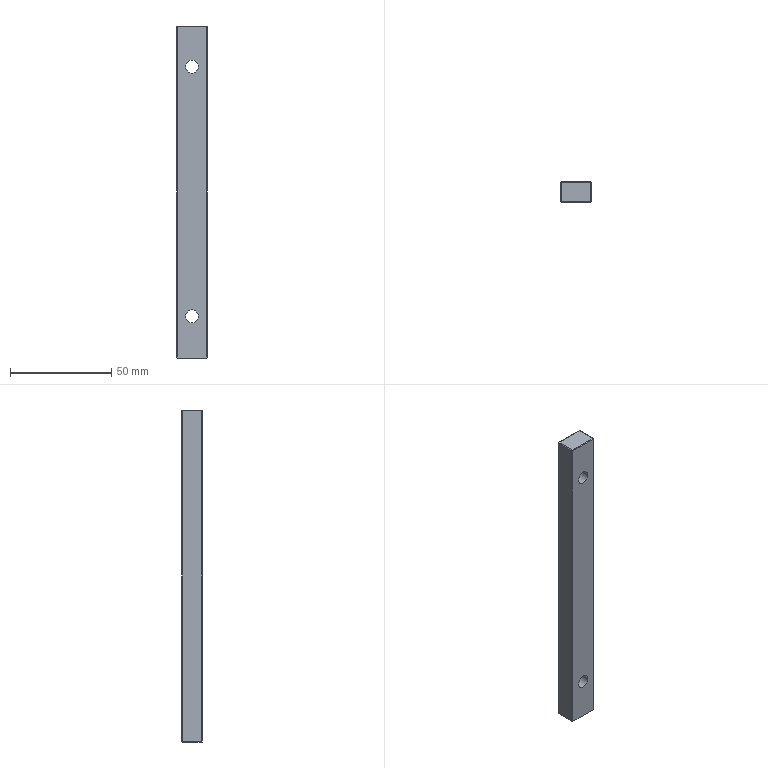Part | NX | 1 solid | 25 faces | box 15 x 10 x 164 mm | volume 23902 mm3 | plane 17 | cylinder 4 | cone 4 | commonest cylinder face diameters 6.5 x4
STEP:
#1=CARTESIAN_POINT('',(0.000000309,-112.2,61.7));
#2=VERTEX_POINT('',#1);
#3=CARTESIAN_POINT('',(0.000000309,-102.8,61.7));
#4=VERTEX_POINT('',#3);
#5=CARTESIAN_POINT('',(0.000000309,-107.5,61.7));
#6=DIRECTION('',(0.,1.,0.));
#7=VECTOR('',#6,1000.);
#8=LINE('',#5,#7);
#9=EDGE_CURVE('',#2,#4,#8,.T.);
#10=ORIENTED_EDGE('',*,*,#9,.F.);
#11=CARTESIAN_POINT('',(0.000000309,-112.2,-101.7));
#12=VERTEX_POINT('',#11);
#13=CARTESIAN_POINT('',(0.000000309,-112.2,-20.));
#14=DIRECTION('',(0.,0.,-1.));
#15=VECTOR('',#14,1000.);
#16=LINE('',#13,#15);
#17=EDGE_CURVE('',#2,#12,#16,.T.);
#18=ORIENTED_EDGE('',*,*,#17,.T.);
#19=CARTESIAN_POINT('',(0.000000309,-102.8,-101.7));
#20=VERTEX_POINT('',#19);
#21=CARTESIAN_POINT('',(0.000000309,-107.5,-101.7));
#22=DIRECTION('',(0.,-1.,0.));
#23=VECTOR('',#22,1000.);
#24=LINE('',#21,#23);
#25=EDGE_CURVE('',#20,#12,#24,.T.);
#26=ORIENTED_EDGE('',*,*,#25,.F.);
#27=CARTESIAN_POINT('',(0.000000309,-102.8,-20.));
#28=DIRECTION('',(0.,0.,1.));
#29=VECTOR('',#28,1000.);
#30=LINE('',#27,#29);
#31=EDGE_CURVE('',#20,#4,#30,.T.);
#32=ORIENTED_EDGE('',*,*,#31,.T.);
#33=EDGE_LOOP('',(#10,#18,#26,#32));
#34=FACE_BOUND('',#33,.T.);
#35=CARTESIAN_POINT('',(0.000000309,-100.5,62.));
#36=DIRECTION('',(1.,0.,0.));
#37=DIRECTION('',(0.,1.,0.));
#38=AXIS2_PLACEMENT_3D('',#35,#36,#37);
#39=PLANE('',#38);
#40=ADVANCED_FACE('',(#34),#39,.T.);
#41=CARTESIAN_POINT('',(-14.7,-102.8,62.));
#42=VERTEX_POINT('',#41);
#43=CARTESIAN_POINT('',(-14.7,-112.2,62.));
#44=VERTEX_POINT('',#43);
#45=CARTESIAN_POINT('',(-14.7,-107.5,62.));
#46=DIRECTION('',(0.,-1.,0.));
#47=VECTOR('',#46,1000.);
#48=LINE('',#45,#47);
#49=EDGE_CURVE('',#42,#44,#48,.T.);
#50=ORIENTED_EDGE('',*,*,#49,.T.);
#51=CARTESIAN_POINT('',(-0.3,-112.2,62.));
#52=VERTEX_POINT('',#51);
#53=CARTESIAN_POINT('',(-7.5,-112.2,62.));
#54=DIRECTION('',(-1.,0.,0.));
#55=VECTOR('',#54,1000.);
#56=LINE('',#53,#55);
#57=EDGE_CURVE('',#52,#44,#56,.T.);
#58=ORIENTED_EDGE('',*,*,#57,.F.);
#59=CARTESIAN_POINT('',(-0.3,-102.8,62.));
#60=VERTEX_POINT('',#59);
#61=CARTESIAN_POINT('',(-0.3,-107.5,62.));
#62=DIRECTION('',(0.,1.,0.));
#63=VECTOR('',#62,1000.);
#64=LINE('',#61,#63);
#65=EDGE_CURVE('',#52,#60,#64,.T.);
#66=ORIENTED_EDGE('',*,*,#65,.T.);
#67=CARTESIAN_POINT('',(-7.5,-102.8,62.));
#68=DIRECTION('',(-1.,0.,0.));
#69=VECTOR('',#68,1000.);
#70=LINE('',#67,#69);
#71=EDGE_CURVE('',#60,#42,#70,.T.);
#72=ORIENTED_EDGE('',*,*,#71,.T.);
#73=EDGE_LOOP('',(#50,#58,#66,#72));
#74=FACE_BOUND('',#73,.T.);
#75=CARTESIAN_POINT('',(-15.,-100.5,62.));
#76=DIRECTION('',(0.,0.,1.));
#77=DIRECTION('',(0.,-1.,0.));
#78=AXIS2_PLACEMENT_3D('',#75,#76,#77);
#79=PLANE('',#78);
#80=ADVANCED_FACE('',(#74),#79,.T.);
#81=CARTESIAN_POINT('',(-15.,-102.8,-101.7));
#82=VERTEX_POINT('',#81);
#83=CARTESIAN_POINT('',(-15.,-112.2,-101.7));
#84=VERTEX_POINT('',#83);
#85=CARTESIAN_POINT('',(-15.,-107.5,-101.7));
#86=DIRECTION('',(0.,-1.,0.));
#87=VECTOR('',#86,1000.);
#88=LINE('',#85,#87);
#89=EDGE_CURVE('',#82,#84,#88,.T.);
#90=ORIENTED_EDGE('',*,*,#89,.T.);
#91=CARTESIAN_POINT('',(-15.,-112.2,61.7));
#92=VERTEX_POINT('',#91);
#93=CARTESIAN_POINT('',(-15.,-112.2,-20.));
#94=DIRECTION('',(0.,0.,-1.));
#95=VECTOR('',#94,1000.);
#96=LINE('',#93,#95);
#97=EDGE_CURVE('',#92,#84,#96,.T.);
#98=ORIENTED_EDGE('',*,*,#97,.F.);
#99=CARTESIAN_POINT('',(-15.,-102.8,61.7));
#100=VERTEX_POINT('',#99);
#101=CARTESIAN_POINT('',(-15.,-107.5,61.7));
#102=DIRECTION('',(0.,-1.,0.));
#103=VECTOR('',#102,1000.);
#104=LINE('',#101,#103);
#105=EDGE_CURVE('',#100,#92,#104,.T.);
#106=ORIENTED_EDGE('',*,*,#105,.F.);
#107=CARTESIAN_POINT('',(-15.,-102.8,-20.));
#108=DIRECTION('',(0.,0.,-1.));
#109=VECTOR('',#108,1000.);
#110=LINE('',#107,#109);
#111=EDGE_CURVE('',#100,#82,#110,.T.);
#112=ORIENTED_EDGE('',*,*,#111,.T.);
#113=EDGE_LOOP('',(#90,#98,#106,#112));
#114=FACE_BOUND('',#113,.T.);
#115=CARTESIAN_POINT('',(-15.,-100.5,-102.));
#116=DIRECTION('',(-1.,0.,0.));
#117=DIRECTION('',(0.,0.,1.));
#118=AXIS2_PLACEMENT_3D('',#115,#116,#117);
#119=PLANE('',#118);
#120=ADVANCED_FACE('',(#114),#119,.T.);
#121=CARTESIAN_POINT('',(-14.7,-102.8,-102.));
#122=VERTEX_POINT('',#121);
#123=CARTESIAN_POINT('',(-0.3,-102.8,-102.));
#124=VERTEX_POINT('',#123);
#125=CARTESIAN_POINT('',(-7.5,-102.8,-102.));
#126=DIRECTION('',(1.,0.,0.));
#127=VECTOR('',#126,1000.);
#128=LINE('',#125,#127);
#129=EDGE_CURVE('',#122,#124,#128,.T.);
#130=ORIENTED_EDGE('',*,*,#129,.T.);
#131=CARTESIAN_POINT('',(-0.3,-112.5,-102.));
#132=VERTEX_POINT('',#131);
#133=CARTESIAN_POINT('',(-0.3,-107.5,-102.));
#134=DIRECTION('',(0.,-1.,0.));
#135=VECTOR('',#134,1000.);
#136=LINE('',#133,#135);
#137=EDGE_CURVE('',#124,#132,#136,.T.);
#138=ORIENTED_EDGE('',*,*,#137,.T.);
#139=CARTESIAN_POINT('',(-14.7,-112.5,-102.));
#140=VERTEX_POINT('',#139);
#141=CARTESIAN_POINT('',(-105.,-112.5,-102.));
#142=DIRECTION('',(1.,0.,0.));
#143=VECTOR('',#142,1000.);
#144=LINE('',#141,#143);
#145=EDGE_CURVE('',#140,#132,#144,.T.);
#146=ORIENTED_EDGE('',*,*,#145,.F.);
#147=CARTESIAN_POINT('',(-14.7,-107.5,-102.));
#148=DIRECTION('',(0.,-1.,0.));
#149=VECTOR('',#148,1000.);
#150=LINE('',#147,#149);
#151=EDGE_CURVE('',#122,#140,#150,.T.);
#152=ORIENTED_EDGE('',*,*,#151,.F.);
#153=EDGE_LOOP('',(#130,#138,#146,#152));
#154=FACE_BOUND('',#153,.T.);
#155=CARTESIAN_POINT('',(-4.,-100.5,-102.));
#156=DIRECTION('',(0.,0.,-1.));
#157=DIRECTION('',(-1.,0.,0.));
#158=AXIS2_PLACEMENT_3D('',#155,#156,#157);
#159=PLANE('',#158);
#160=ADVANCED_FACE('',(#154),#159,.T.);
#161=CARTESIAN_POINT('',(-4.25,-102.7,-81.438));
#162=VERTEX_POINT('',#161);
#163=CARTESIAN_POINT('',(-10.75,-102.7,-81.438));
#164=VERTEX_POINT('',#163);
#165=CARTESIAN_POINT('',(-7.5,-102.7,-81.438));
#166=DIRECTION('',(0.,1.,0.));
#167=DIRECTION('',(-1.,0.,0.));
#168=AXIS2_PLACEMENT_3D('',#165,#166,#167);
#169=CIRCLE('',#168,3.25);
#170=EDGE_CURVE('',#162,#164,#169,.T.);
#171=ORIENTED_EDGE('',*,*,#170,.T.);
#172=CARTESIAN_POINT('',(-10.75,-112.5,-81.438));
#173=VERTEX_POINT('',#172);
#174=CARTESIAN_POINT('',(-10.75,-102.5,-81.438));
#175=DIRECTION('',(0.,1.,0.));
#176=VECTOR('',#175,1000.);
#177=LINE('',#174,#176);
#178=EDGE_CURVE('',#164,#173,#177,.F.);
#179=ORIENTED_EDGE('',*,*,#178,.T.);
#180=CARTESIAN_POINT('',(-4.25,-112.5,-81.438));
#181=VERTEX_POINT('',#180);
#182=CARTESIAN_POINT('',(-7.5,-112.5,-81.438));
#183=DIRECTION('',(0.,1.,0.));
#184=DIRECTION('',(-1.,0.,0.));
#185=AXIS2_PLACEMENT_3D('',#182,#183,#184);
#186=CIRCLE('',#185,3.25);
#187=EDGE_CURVE('',#181,#173,#186,.T.);
#188=ORIENTED_EDGE('',*,*,#187,.F.);
#189=CARTESIAN_POINT('',(-4.25,-102.5,-81.438));
#190=DIRECTION('',(0.,1.,0.));
#191=VECTOR('',#190,1000.);
#192=LINE('',#189,#191);
#193=EDGE_CURVE('',#162,#181,#192,.F.);
#194=ORIENTED_EDGE('',*,*,#193,.F.);
#195=EDGE_LOOP('',(#171,#179,#188,#194));
#196=FACE_BOUND('',#195,.T.);
#197=CARTESIAN_POINT('',(-7.5,-102.5,-81.438));
#198=DIRECTION('',(0.,1.,0.));
#199=DIRECTION('',(-1.,0.,0.));
#200=AXIS2_PLACEMENT_3D('',#197,#198,#199);
#201=CYLINDRICAL_SURFACE('',#200,3.25);
#202=ADVANCED_FACE('',(#196),#201,.F.);
#203=ORIENTED_EDGE('',*,*,#170,.F.);
#204=CARTESIAN_POINT('',(-4.05,-102.5,-81.438));
#205=VERTEX_POINT('',#204);
#206=CARTESIAN_POINT('',(-4.25,-102.7,-81.438));
#207=DIRECTION('',(0.7071,0.7071,0.));
#208=VECTOR('',#207,1000.);
#209=LINE('',#206,#208);
#210=EDGE_CURVE('',#205,#162,#209,.F.);
#211=ORIENTED_EDGE('',*,*,#210,.F.);
#212=CARTESIAN_POINT('',(-10.95,-102.5,-81.438));
#213=VERTEX_POINT('',#212);
#214=CARTESIAN_POINT('',(-7.5,-102.5,-81.438));
#215=DIRECTION('',(0.,1.,0.));
#216=DIRECTION('',(-1.,0.,0.));
#217=AXIS2_PLACEMENT_3D('',#214,#215,#216);
#218=CIRCLE('',#217,3.45);
#219=EDGE_CURVE('',#205,#213,#218,.T.);
#220=ORIENTED_EDGE('',*,*,#219,.T.);
#221=CARTESIAN_POINT('',(-10.75,-102.7,-81.438));
#222=DIRECTION('',(-0.7071,0.7071,0.));
#223=VECTOR('',#222,1000.);
#224=LINE('',#221,#223);
#225=EDGE_CURVE('',#213,#164,#224,.F.);
#226=ORIENTED_EDGE('',*,*,#225,.T.);
#227=EDGE_LOOP('',(#203,#211,#220,#226));
#228=FACE_BOUND('',#227,.T.);
#229=CARTESIAN_POINT('',(-7.5,-102.7,-81.438));
#230=DIRECTION('',(0.,1.,0.));
#231=DIRECTION('',(-1.,0.,0.));
#232=AXIS2_PLACEMENT_3D('',#229,#230,#231);
#233=CONICAL_SURFACE('',#232,3.25,0.7854);
#234=ADVANCED_FACE('',(#228),#233,.F.);
#235=ORIENTED_EDGE('',*,*,#89,.F.);
#236=CARTESIAN_POINT('',(-14.85,-102.65,-101.85));
#237=VERTEX_POINT('',#236);
#238=CARTESIAN_POINT('',(-12.7,-100.5,-104.));
#239=DIRECTION('',(0.5774,0.5774,-0.5774));
#240=VECTOR('',#239,1000.);
#241=LINE('',#238,#240);
#242=EDGE_CURVE('',#82,#237,#241,.T.);
#243=ORIENTED_EDGE('',*,*,#242,.T.);
#244=CARTESIAN_POINT('',(-17.,-100.5,-99.7));
#245=DIRECTION('',(0.5774,-0.5774,-0.5774));
#246=VECTOR('',#245,1000.);
#247=LINE('',#244,#246);
#248=EDGE_CURVE('',#237,#122,#247,.T.);
#249=ORIENTED_EDGE('',*,*,#248,.T.);
#250=ORIENTED_EDGE('',*,*,#151,.T.);
#251=CARTESIAN_POINT('',(-26.7,-100.5,-90.));
#252=DIRECTION('',(-0.5774,0.5774,0.5774));
#253=VECTOR('',#252,1000.);
#254=LINE('',#251,#253);
#255=EDGE_CURVE('',#140,#84,#254,.T.);
#256=ORIENTED_EDGE('',*,*,#255,.T.);
#257=EDGE_LOOP('',(#235,#243,#249,#250,#256));
#258=FACE_BOUND('',#257,.T.);
#259=CARTESIAN_POINT('',(-14.85,-107.5,-101.85));
#260=DIRECTION('',(-0.7071,0.,-0.7071));
#261=DIRECTION('',(-0.7071,0.,0.7071));
#262=AXIS2_PLACEMENT_3D('',#259,#260,#261);
#263=PLANE('',#262);
#264=ADVANCED_FACE('',(#258),#263,.T.);
#265=ORIENTED_EDGE('',*,*,#25,.T.);
#266=CARTESIAN_POINT('',(81.95,-30.25,-19.75));
#267=DIRECTION('',(-0.5774,-0.5774,-0.5774));
#268=VECTOR('',#267,1000.);
#269=LINE('',#266,#268);
#270=EDGE_CURVE('',#12,#132,#269,.T.);
#271=ORIENTED_EDGE('',*,*,#270,.T.);
#272=ORIENTED_EDGE('',*,*,#137,.F.);
#273=CARTESIAN_POINT('',(-0.15,-102.65,-101.85));
#274=VERTEX_POINT('',#273);
#275=CARTESIAN_POINT('',(2.,-100.5,-99.7));
#276=DIRECTION('',(-0.5774,-0.5774,-0.5774));
#277=VECTOR('',#276,1000.);
#278=LINE('',#275,#277);
#279=EDGE_CURVE('',#274,#124,#278,.T.);
#280=ORIENTED_EDGE('',*,*,#279,.F.);
#281=CARTESIAN_POINT('',(81.95,-184.75,-19.75));
#282=DIRECTION('',(0.5774,-0.5774,0.5774));
#283=VECTOR('',#282,1000.);
#284=LINE('',#281,#283);
#285=EDGE_CURVE('',#274,#20,#284,.T.);
#286=ORIENTED_EDGE('',*,*,#285,.T.);
#287=EDGE_LOOP('',(#265,#271,#272,#280,#286));
#288=FACE_BOUND('',#287,.T.);
#289=CARTESIAN_POINT('',(-0.15,-107.5,-101.85));
#290=DIRECTION('',(-0.7071,0.,0.7071));
#291=DIRECTION('',(0.,1.,0.));
#292=AXIS2_PLACEMENT_3D('',#289,#290,#291);
#293=PLANE('',#292);
#294=ADVANCED_FACE('',(#288),#293,.F.);
#295=ORIENTED_EDGE('',*,*,#49,.F.);
#296=CARTESIAN_POINT('',(-14.85,-102.65,61.85));
#297=VERTEX_POINT('',#296);
#298=CARTESIAN_POINT('',(-17.,-100.5,59.7));
#299=DIRECTION('',(0.5774,-0.5774,0.5774));
#300=VECTOR('',#299,1000.);
#301=LINE('',#298,#300);
#302=EDGE_CURVE('',#297,#42,#301,.T.);
#303=ORIENTED_EDGE('',*,*,#302,.F.);
#304=CARTESIAN_POINT('',(-96.45,-184.25,-19.75));
#305=DIRECTION('',(-0.5774,-0.5774,-0.5774));
#306=VECTOR('',#305,1000.);
#307=LINE('',#304,#306);
#308=EDGE_CURVE('',#297,#100,#307,.T.);
#309=ORIENTED_EDGE('',*,*,#308,.T.);
#310=ORIENTED_EDGE('',*,*,#105,.T.);
#311=CARTESIAN_POINT('',(-14.85,-112.35,61.85));
#312=VERTEX_POINT('',#311);
#313=CARTESIAN_POINT('',(-96.45,-30.75,-19.75));
#314=DIRECTION('',(-0.5774,0.5774,-0.5774));
#315=VECTOR('',#314,1000.);
#316=LINE('',#313,#315);
#317=EDGE_CURVE('',#312,#92,#316,.T.);
#318=ORIENTED_EDGE('',*,*,#317,.F.);
#319=CARTESIAN_POINT('',(-3.,-100.5,73.7));
#320=DIRECTION('',(0.5774,0.5774,0.5774));
#321=VECTOR('',#320,1000.);
#322=LINE('',#319,#321);
#323=EDGE_CURVE('',#312,#44,#322,.T.);
#324=ORIENTED_EDGE('',*,*,#323,.T.);
#325=EDGE_LOOP('',(#295,#303,#309,#310,#318,#324));
#326=FACE_BOUND('',#325,.T.);
#327=CARTESIAN_POINT('',(-14.85,-107.5,61.85));
#328=DIRECTION('',(-0.7071,0.,0.7071));
#329=DIRECTION('',(0.,1.,0.));
#330=AXIS2_PLACEMENT_3D('',#327,#328,#329);
#331=PLANE('',#330);
#332=ADVANCED_FACE('',(#326),#331,.T.);
#333=ORIENTED_EDGE('',*,*,#9,.T.);
#334=CARTESIAN_POINT('',(-0.15,-102.65,61.85));
#335=VERTEX_POINT('',#334);
#336=CARTESIAN_POINT('',(-2.3,-100.5,64.));
#337=DIRECTION('',(0.5774,-0.5774,-0.5774));
#338=VECTOR('',#337,1000.);
#339=LINE('',#336,#338);
#340=EDGE_CURVE('',#335,#4,#339,.T.);
#341=ORIENTED_EDGE('',*,*,#340,.F.);
#342=CARTESIAN_POINT('',(2.,-100.5,59.7));
#343=DIRECTION('',(0.5774,0.5774,-0.5774));
#344=VECTOR('',#343,1000.);
#345=LINE('',#342,#344);
#346=EDGE_CURVE('',#60,#335,#345,.T.);
#347=ORIENTED_EDGE('',*,*,#346,.F.);
#348=ORIENTED_EDGE('',*,*,#65,.F.);
#349=CARTESIAN_POINT('',(-0.15,-112.35,61.85));
#350=VERTEX_POINT('',#349);
#351=CARTESIAN_POINT('',(-12.,-100.5,73.7));
#352=DIRECTION('',(-0.5774,0.5774,0.5774));
#353=VECTOR('',#352,1000.);
#354=LINE('',#351,#353);
#355=EDGE_CURVE('',#350,#52,#354,.T.);
#356=ORIENTED_EDGE('',*,*,#355,.F.);
#357=CARTESIAN_POINT('',(11.7,-100.5,50.));
#358=DIRECTION('',(-0.5774,-0.5774,0.5774));
#359=VECTOR('',#358,1000.);
#360=LINE('',#357,#359);
#361=EDGE_CURVE('',#2,#350,#360,.T.);
#362=ORIENTED_EDGE('',*,*,#361,.F.);
#363=EDGE_LOOP('',(#333,#341,#347,#348,#356,#362));
#364=FACE_BOUND('',#363,.T.);
#365=CARTESIAN_POINT('',(-0.15,-107.5,61.85));
#366=DIRECTION('',(-0.7071,0.,-0.7071));
#367=DIRECTION('',(-0.7071,0.,0.7071));
#368=AXIS2_PLACEMENT_3D('',#365,#366,#367);
#369=PLANE('',#368);
#370=ADVANCED_FACE('',(#364),#369,.F.);
#371=ORIENTED_EDGE('',*,*,#178,.F.);
#372=CARTESIAN_POINT('',(-7.5,-102.7,-81.438));
#373=DIRECTION('',(0.,1.,0.));
#374=DIRECTION('',(-1.,0.,0.));
#375=AXIS2_PLACEMENT_3D('',#372,#373,#374);
#376=CIRCLE('',#375,3.25);
#377=EDGE_CURVE('',#164,#162,#376,.T.);
#378=ORIENTED_EDGE('',*,*,#377,.T.);
#379=ORIENTED_EDGE('',*,*,#193,.T.);
#380=CARTESIAN_POINT('',(-7.5,-112.5,-81.438));
#381=DIRECTION('',(0.,1.,0.));
#382=DIRECTION('',(-1.,0.,0.));
#383=AXIS2_PLACEMENT_3D('',#380,#381,#382);
#384=CIRCLE('',#383,3.25);
#385=EDGE_CURVE('',#173,#181,#384,.T.);
#386=ORIENTED_EDGE('',*,*,#385,.F.);
#387=EDGE_LOOP('',(#371,#378,#379,#386));
#388=FACE_BOUND('',#387,.T.);
#389=CARTESIAN_POINT('',(-7.5,-102.5,-81.438));
#390=DIRECTION('',(0.,1.,0.));
#391=DIRECTION('',(-1.,0.,0.));
#392=AXIS2_PLACEMENT_3D('',#389,#390,#391);
#393=CYLINDRICAL_SURFACE('',#392,3.25);
#394=ADVANCED_FACE('',(#388),#393,.F.);
#395=ORIENTED_EDGE('',*,*,#225,.F.);
#396=CARTESIAN_POINT('',(-7.5,-102.5,-81.438));
#397=DIRECTION('',(0.,1.,0.));
#398=DIRECTION('',(-1.,0.,0.));
#399=AXIS2_PLACEMENT_3D('',#396,#397,#398);
#400=CIRCLE('',#399,3.45);
#401=EDGE_CURVE('',#213,#205,#400,.T.);
#402=ORIENTED_EDGE('',*,*,#401,.T.);
#403=ORIENTED_EDGE('',*,*,#210,.T.);
#404=ORIENTED_EDGE('',*,*,#377,.F.);
#405=EDGE_LOOP('',(#395,#402,#403,#404));
#406=FACE_BOUND('',#405,.T.);
#407=CARTESIAN_POINT('',(-7.5,-102.7,-81.438));
#408=DIRECTION('',(0.,1.,0.));
#409=DIRECTION('',(-1.,0.,0.));
#410=AXIS2_PLACEMENT_3D('',#407,#408,#409);
#411=CONICAL_SURFACE('',#410,3.25,0.7854);
#412=ADVANCED_FACE('',(#406),#411,.F.);
#413=CARTESIAN_POINT('',(-0.3,-112.5,61.7));
#414=VERTEX_POINT('',#413);
#415=CARTESIAN_POINT('',(-14.7,-112.5,61.7));
#416=VERTEX_POINT('',#415);
#417=CARTESIAN_POINT('',(-7.5,-112.5,61.7));
#418=DIRECTION('',(-1.,0.,0.));
#419=VECTOR('',#418,1000.);
#420=LINE('',#417,#419);
#421=EDGE_CURVE('',#414,#416,#420,.T.);
#422=ORIENTED_EDGE('',*,*,#421,.T.);
#423=CARTESIAN_POINT('',(-14.7,-112.5,-20.));
#424=DIRECTION('',(0.,0.,-1.));
#425=VECTOR('',#424,1000.);
#426=LINE('',#423,#425);
#427=EDGE_CURVE('',#416,#140,#426,.T.);
#428=ORIENTED_EDGE('',*,*,#427,.T.);
#429=ORIENTED_EDGE('',*,*,#145,.T.);
#430=CARTESIAN_POINT('',(-0.3,-112.5,-20.));
#431=DIRECTION('',(0.,0.,-1.));
#432=VECTOR('',#431,1000.);
#433=LINE('',#430,#432);
#434=EDGE_CURVE('',#414,#132,#433,.T.);
#435=ORIENTED_EDGE('',*,*,#434,.F.);
#436=EDGE_LOOP('',(#422,#428,#429,#435));
#437=FACE_BOUND('',#436,.T.);
#438=ORIENTED_EDGE('',*,*,#187,.T.);
#439=ORIENTED_EDGE('',*,*,#385,.T.);
#440=EDGE_LOOP('',(#438,#439));
#441=FACE_BOUND('',#440,.T.);
#442=CARTESIAN_POINT('',(-4.25,-112.5,41.937));
#443=VERTEX_POINT('',#442);
#444=CARTESIAN_POINT('',(-10.75,-112.5,41.937));
#445=VERTEX_POINT('',#444);
#446=CARTESIAN_POINT('',(-7.5,-112.5,41.937));
#447=DIRECTION('',(0.,1.,0.));
#448=DIRECTION('',(-1.,0.,0.));
#449=AXIS2_PLACEMENT_3D('',#446,#447,#448);
#450=CIRCLE('',#449,3.25);
#451=EDGE_CURVE('',#443,#445,#450,.T.);
#452=ORIENTED_EDGE('',*,*,#451,.T.);
#453=CARTESIAN_POINT('',(-7.5,-112.5,41.937));
#454=DIRECTION('',(0.,1.,0.));
#455=DIRECTION('',(-1.,0.,0.));
#456=AXIS2_PLACEMENT_3D('',#453,#454,#455);
#457=CIRCLE('',#456,3.25);
#458=EDGE_CURVE('',#445,#443,#457,.T.);
#459=ORIENTED_EDGE('',*,*,#458,.T.);
#460=EDGE_LOOP('',(#452,#459));
#461=FACE_BOUND('',#460,.T.);
#462=CARTESIAN_POINT('',(-105.,-112.5,-19.75));
#463=DIRECTION('',(0.,1.,0.));
#464=DIRECTION('',(0.,0.,-1.));
#465=AXIS2_PLACEMENT_3D('',#462,#463,#464);
#466=PLANE('',#465);
#467=ADVANCED_FACE('',(#437,#441,#461),#466,.F.);
#468=CARTESIAN_POINT('',(-4.25,-102.7,41.937));
#469=VERTEX_POINT('',#468);
#470=CARTESIAN_POINT('',(-10.75,-102.7,41.937));
#471=VERTEX_POINT('',#470);
#472=CARTESIAN_POINT('',(-7.5,-102.7,41.937));
#473=DIRECTION('',(0.,1.,0.));
#474=DIRECTION('',(-1.,0.,0.));
#475=AXIS2_PLACEMENT_3D('',#472,#473,#474);
#476=CIRCLE('',#475,3.25);
#477=EDGE_CURVE('',#469,#471,#476,.T.);
#478=ORIENTED_EDGE('',*,*,#477,.T.);
#479=CARTESIAN_POINT('',(-10.75,-102.5,41.937));
#480=DIRECTION('',(0.,1.,0.));
#481=VECTOR('',#480,1000.);
#482=LINE('',#479,#481);
#483=EDGE_CURVE('',#471,#445,#482,.F.);
#484=ORIENTED_EDGE('',*,*,#483,.T.);
#485=ORIENTED_EDGE('',*,*,#451,.F.);
#486=CARTESIAN_POINT('',(-4.25,-102.5,41.937));
#487=DIRECTION('',(0.,1.,0.));
#488=VECTOR('',#487,1000.);
#489=LINE('',#486,#488);
#490=EDGE_CURVE('',#469,#443,#489,.F.);
#491=ORIENTED_EDGE('',*,*,#490,.F.);
#492=EDGE_LOOP('',(#478,#484,#485,#491));
#493=FACE_BOUND('',#492,.T.);
#494=CARTESIAN_POINT('',(-7.5,-102.5,41.937));
#495=DIRECTION('',(0.,1.,0.));
#496=DIRECTION('',(-1.,0.,0.));
#497=AXIS2_PLACEMENT_3D('',#494,#495,#496);
#498=CYLINDRICAL_SURFACE('',#497,3.25);
#499=ADVANCED_FACE('',(#493),#498,.F.);
#500=ORIENTED_EDGE('',*,*,#477,.F.);
#501=CARTESIAN_POINT('',(-4.05,-102.5,41.937));
#502=VERTEX_POINT('',#501);
#503=CARTESIAN_POINT('',(-4.25,-102.7,41.937));
#504=DIRECTION('',(0.7071,0.7071,0.));
#505=VECTOR('',#504,1000.);
#506=LINE('',#503,#505);
#507=EDGE_CURVE('',#502,#469,#506,.F.);
#508=ORIENTED_EDGE('',*,*,#507,.F.);
#509=CARTESIAN_POINT('',(-10.95,-102.5,41.937));
#510=VERTEX_POINT('',#509);
#511=CARTESIAN_POINT('',(-7.5,-102.5,41.937));
#512=DIRECTION('',(0.,1.,0.));
#513=DIRECTION('',(-1.,0.,0.));
#514=AXIS2_PLACEMENT_3D('',#511,#512,#513);
#515=CIRCLE('',#514,3.45);
#516=EDGE_CURVE('',#502,#510,#515,.T.);
#517=ORIENTED_EDGE('',*,*,#516,.T.);
#518=CARTESIAN_POINT('',(-10.75,-102.7,41.937));
#519=DIRECTION('',(-0.7071,0.7071,0.));
#520=VECTOR('',#519,1000.);
#521=LINE('',#518,#520);
#522=EDGE_CURVE('',#510,#471,#521,.F.);
#523=ORIENTED_EDGE('',*,*,#522,.T.);
#524=EDGE_LOOP('',(#500,#508,#517,#523));
#525=FACE_BOUND('',#524,.T.);
#526=CARTESIAN_POINT('',(-7.5,-102.7,41.937));
#527=DIRECTION('',(0.,1.,0.));
#528=DIRECTION('',(-1.,0.,0.));
#529=AXIS2_PLACEMENT_3D('',#526,#527,#528);
#530=CONICAL_SURFACE('',#529,3.25,0.7854);
#531=ADVANCED_FACE('',(#525),#530,.F.);
#532=ORIENTED_EDGE('',*,*,#427,.F.);
#533=CARTESIAN_POINT('',(-26.7,-100.5,73.7));
#534=DIRECTION('',(-0.5774,0.5774,0.5774));
#535=VECTOR('',#534,1000.);
#536=LINE('',#533,#535);
#537=EDGE_CURVE('',#416,#312,#536,.T.);
#538=ORIENTED_EDGE('',*,*,#537,.T.);
#539=ORIENTED_EDGE('',*,*,#317,.T.);
#540=ORIENTED_EDGE('',*,*,#97,.T.);
#541=ORIENTED_EDGE('',*,*,#255,.F.);
#542=EDGE_LOOP('',(#532,#538,#539,#540,#541));
#543=FACE_BOUND('',#542,.T.);
#544=CARTESIAN_POINT('',(-14.85,-112.35,-20.));
#545=DIRECTION('',(-0.7071,-0.7071,0.));
#546=DIRECTION('',(-0.7071,0.7071,0.));
#547=AXIS2_PLACEMENT_3D('',#544,#545,#546);
#548=PLANE('',#547);
#549=ADVANCED_FACE('',(#543),#548,.T.);
#550=ORIENTED_EDGE('',*,*,#434,.T.);
#551=ORIENTED_EDGE('',*,*,#270,.F.);
#552=ORIENTED_EDGE('',*,*,#17,.F.);
#553=ORIENTED_EDGE('',*,*,#361,.T.);
#554=CARTESIAN_POINT('',(11.7,-100.5,73.7));
#555=DIRECTION('',(0.5774,0.5774,0.5774));
#556=VECTOR('',#555,1000.);
#557=LINE('',#554,#556);
#558=EDGE_CURVE('',#414,#350,#557,.T.);
#559=ORIENTED_EDGE('',*,*,#558,.F.);
#560=EDGE_LOOP('',(#550,#551,#552,#553,#559));
#561=FACE_BOUND('',#560,.T.);
#562=CARTESIAN_POINT('',(-0.15,-112.35,-20.));
#563=DIRECTION('',(-0.7071,0.7071,0.));
#564=DIRECTION('',(0.,0.,1.));
#565=AXIS2_PLACEMENT_3D('',#562,#563,#564);
#566=PLANE('',#565);
#567=ADVANCED_FACE('',(#561),#566,.F.);
#568=ORIENTED_EDGE('',*,*,#421,.F.);
#569=ORIENTED_EDGE('',*,*,#558,.T.);
#570=ORIENTED_EDGE('',*,*,#355,.T.);
#571=ORIENTED_EDGE('',*,*,#57,.T.);
#572=ORIENTED_EDGE('',*,*,#323,.F.);
#573=ORIENTED_EDGE('',*,*,#537,.F.);
#574=EDGE_LOOP('',(#568,#569,#570,#571,#572,#573));
#575=FACE_BOUND('',#574,.T.);
#576=CARTESIAN_POINT('',(-7.5,-112.35,61.85));
#577=DIRECTION('',(0.,-0.7071,0.7071));
#578=DIRECTION('',(-1.,0.,0.));
#579=AXIS2_PLACEMENT_3D('',#576,#577,#578);
#580=PLANE('',#579);
#581=ADVANCED_FACE('',(#575),#580,.T.);
#582=ORIENTED_EDGE('',*,*,#483,.F.);
#583=CARTESIAN_POINT('',(-7.5,-102.7,41.937));
#584=DIRECTION('',(0.,1.,0.));
#585=DIRECTION('',(-1.,0.,0.));
#586=AXIS2_PLACEMENT_3D('',#583,#584,#585);
#587=CIRCLE('',#586,3.25);
#588=EDGE_CURVE('',#471,#469,#587,.T.);
#589=ORIENTED_EDGE('',*,*,#588,.T.);
#590=ORIENTED_EDGE('',*,*,#490,.T.);
#591=ORIENTED_EDGE('',*,*,#458,.F.);
#592=EDGE_LOOP('',(#582,#589,#590,#591));
#593=FACE_BOUND('',#592,.T.);
#594=CARTESIAN_POINT('',(-7.5,-102.5,41.937));
#595=DIRECTION('',(0.,1.,0.));
#596=DIRECTION('',(-1.,0.,0.));
#597=AXIS2_PLACEMENT_3D('',#594,#595,#596);
#598=CYLINDRICAL_SURFACE('',#597,3.25);
#599=ADVANCED_FACE('',(#593),#598,.F.);
#600=ORIENTED_EDGE('',*,*,#522,.F.);
#601=CARTESIAN_POINT('',(-7.5,-102.5,41.937));
#602=DIRECTION('',(0.,1.,0.));
#603=DIRECTION('',(-1.,0.,0.));
#604=AXIS2_PLACEMENT_3D('',#601,#602,#603);
#605=CIRCLE('',#604,3.45);
#606=EDGE_CURVE('',#510,#502,#605,.T.);
#607=ORIENTED_EDGE('',*,*,#606,.T.);
#608=ORIENTED_EDGE('',*,*,#507,.T.);
#609=ORIENTED_EDGE('',*,*,#588,.F.);
#610=EDGE_LOOP('',(#600,#607,#608,#609));
#611=FACE_BOUND('',#610,.T.);
#612=CARTESIAN_POINT('',(-7.5,-102.7,41.937));
#613=DIRECTION('',(0.,1.,0.));
#614=DIRECTION('',(-1.,0.,0.));
#615=AXIS2_PLACEMENT_3D('',#612,#613,#614);
#616=CONICAL_SURFACE('',#615,3.25,0.7854);
#617=ADVANCED_FACE('',(#611),#616,.F.);
#618=CARTESIAN_POINT('',(-0.3,-102.5,61.7));
#619=VERTEX_POINT('',#618);
#620=CARTESIAN_POINT('',(-14.7,-102.5,61.7));
#621=VERTEX_POINT('',#620);
#622=CARTESIAN_POINT('',(-7.5,-102.5,61.7));
#623=DIRECTION('',(-1.,0.,0.));
#624=VECTOR('',#623,1000.);
#625=LINE('',#622,#624);
#626=EDGE_CURVE('',#619,#621,#625,.T.);
#627=ORIENTED_EDGE('',*,*,#626,.F.);
#628=CARTESIAN_POINT('',(-0.3,-102.5,-101.7));
#629=VERTEX_POINT('',#628);
#630=CARTESIAN_POINT('',(-0.3,-102.5,-20.));
#631=DIRECTION('',(0.,0.,1.));
#632=VECTOR('',#631,1000.);
#633=LINE('',#630,#632);
#634=EDGE_CURVE('',#629,#619,#633,.T.);
#635=ORIENTED_EDGE('',*,*,#634,.F.);
#636=CARTESIAN_POINT('',(-14.7,-102.5,-101.7));
#637=VERTEX_POINT('',#636);
#638=CARTESIAN_POINT('',(-7.5,-102.5,-101.7));
#639=DIRECTION('',(1.,0.,0.));
#640=VECTOR('',#639,1000.);
#641=LINE('',#638,#640);
#642=EDGE_CURVE('',#637,#629,#641,.T.);
#643=ORIENTED_EDGE('',*,*,#642,.F.);
#644=CARTESIAN_POINT('',(-14.7,-102.5,-20.));
#645=DIRECTION('',(0.,0.,-1.));
#646=VECTOR('',#645,1000.);
#647=LINE('',#644,#646);
#648=EDGE_CURVE('',#621,#637,#647,.T.);
#649=ORIENTED_EDGE('',*,*,#648,.F.);
#650=EDGE_LOOP('',(#627,#635,#643,#649));
#651=FACE_BOUND('',#650,.T.);
#652=ORIENTED_EDGE('',*,*,#516,.F.);
#653=ORIENTED_EDGE('',*,*,#606,.F.);
#654=EDGE_LOOP('',(#652,#653));
#655=FACE_BOUND('',#654,.T.);
#656=ORIENTED_EDGE('',*,*,#219,.F.);
#657=ORIENTED_EDGE('',*,*,#401,.F.);
#658=EDGE_LOOP('',(#656,#657));
#659=FACE_BOUND('',#658,.T.);
#660=CARTESIAN_POINT('',(-105.,-102.5,-19.75));
#661=DIRECTION('',(0.,1.,0.));
#662=DIRECTION('',(0.,0.,-1.));
#663=AXIS2_PLACEMENT_3D('',#660,#661,#662);
#664=PLANE('',#663);
#665=ADVANCED_FACE('',(#651,#655,#659),#664,.T.);
#666=ORIENTED_EDGE('',*,*,#642,.T.);
#667=CARTESIAN_POINT('',(-2.3,-100.5,-99.7));
#668=DIRECTION('',(0.5774,-0.5774,-0.5774));
#669=VECTOR('',#668,1000.);
#670=LINE('',#667,#669);
#671=EDGE_CURVE('',#629,#274,#670,.T.);
#672=ORIENTED_EDGE('',*,*,#671,.T.);
#673=ORIENTED_EDGE('',*,*,#279,.T.);
#674=ORIENTED_EDGE('',*,*,#129,.F.);
#675=ORIENTED_EDGE('',*,*,#248,.F.);
#676=CARTESIAN_POINT('',(-12.7,-100.5,-99.7));
#677=DIRECTION('',(0.5774,0.5774,0.5774));
#678=VECTOR('',#677,1000.);
#679=LINE('',#676,#678);
#680=EDGE_CURVE('',#237,#637,#679,.T.);
#681=ORIENTED_EDGE('',*,*,#680,.T.);
#682=EDGE_LOOP('',(#666,#672,#673,#674,#675,#681));
#683=FACE_BOUND('',#682,.T.);
#684=CARTESIAN_POINT('',(-7.5,-102.65,-101.85));
#685=DIRECTION('',(0.,-0.7071,0.7071));
#686=DIRECTION('',(-1.,0.,0.));
#687=AXIS2_PLACEMENT_3D('',#684,#685,#686);
#688=PLANE('',#687);
#689=ADVANCED_FACE('',(#683),#688,.F.);
#690=ORIENTED_EDGE('',*,*,#648,.T.);
#691=ORIENTED_EDGE('',*,*,#680,.F.);
#692=ORIENTED_EDGE('',*,*,#242,.F.);
#693=ORIENTED_EDGE('',*,*,#111,.F.);
#694=ORIENTED_EDGE('',*,*,#308,.F.);
#695=CARTESIAN_POINT('',(-12.7,-100.5,59.7));
#696=DIRECTION('',(0.5774,0.5774,-0.5774));
#697=VECTOR('',#696,1000.);
#698=LINE('',#695,#697);
#699=EDGE_CURVE('',#297,#621,#698,.T.);
#700=ORIENTED_EDGE('',*,*,#699,.T.);
#701=EDGE_LOOP('',(#690,#691,#692,#693,#694,#700));
#702=FACE_BOUND('',#701,.T.);
#703=CARTESIAN_POINT('',(-14.85,-102.65,-20.));
#704=DIRECTION('',(0.7071,-0.7071,0.));
#705=DIRECTION('',(0.,0.,-1.));
#706=AXIS2_PLACEMENT_3D('',#703,#704,#705);
#707=PLANE('',#706);
#708=ADVANCED_FACE('',(#702),#707,.F.);
#709=ORIENTED_EDGE('',*,*,#634,.T.);
#710=CARTESIAN_POINT('',(-2.3,-100.5,59.7));
#711=DIRECTION('',(0.5774,-0.5774,0.5774));
#712=VECTOR('',#711,1000.);
#713=LINE('',#710,#712);
#714=EDGE_CURVE('',#619,#335,#713,.T.);
#715=ORIENTED_EDGE('',*,*,#714,.T.);
#716=ORIENTED_EDGE('',*,*,#340,.T.);
#717=ORIENTED_EDGE('',*,*,#31,.F.);
#718=ORIENTED_EDGE('',*,*,#285,.F.);
#719=ORIENTED_EDGE('',*,*,#671,.F.);
#720=EDGE_LOOP('',(#709,#715,#716,#717,#718,#719));
#721=FACE_BOUND('',#720,.T.);
#722=CARTESIAN_POINT('',(-0.15,-102.65,-20.));
#723=DIRECTION('',(-0.7071,-0.7071,0.));
#724=DIRECTION('',(-0.7071,0.7071,0.));
#725=AXIS2_PLACEMENT_3D('',#722,#723,#724);
#726=PLANE('',#725);
#727=ADVANCED_FACE('',(#721),#726,.F.);
#728=ORIENTED_EDGE('',*,*,#626,.T.);
#729=ORIENTED_EDGE('',*,*,#699,.F.);
#730=ORIENTED_EDGE('',*,*,#302,.T.);
#731=ORIENTED_EDGE('',*,*,#71,.F.);
#732=ORIENTED_EDGE('',*,*,#346,.T.);
#733=ORIENTED_EDGE('',*,*,#714,.F.);
#734=EDGE_LOOP('',(#728,#729,#730,#731,#732,#733));
#735=FACE_BOUND('',#734,.T.);
#736=CARTESIAN_POINT('',(-7.5,-102.65,61.85));
#737=DIRECTION('',(0.,-0.7071,-0.7071));
#738=DIRECTION('',(0.,-0.7071,0.7071));
#739=AXIS2_PLACEMENT_3D('',#736,#737,#738);
#740=PLANE('',#739);
#741=ADVANCED_FACE('',(#735),#740,.F.);
#742=CLOSED_SHELL('',(#40,#80,#120,#160,#202,#234,#264,#294,#332,#370,#394,#412,#467,#499,#531,#549,#567,#581,#599,#617,#665,#689,#708,#727,#741));
#743=MANIFOLD_SOLID_BREP('',#742);
#744=(LENGTH_UNIT()NAMED_UNIT(*)SI_UNIT(.MILLI.,.METRE.));
#745=UNCERTAINTY_MEASURE_WITH_UNIT(LENGTH_MEASURE(0.00001),#744,'','');
#746=(NAMED_UNIT(*)PLANE_ANGLE_UNIT()SI_UNIT($,.RADIAN.));
#747=(NAMED_UNIT(*)SI_UNIT($,.STERADIAN.)SOLID_ANGLE_UNIT());
#748=(GEOMETRIC_REPRESENTATION_CONTEXT(3)GLOBAL_UNCERTAINTY_ASSIGNED_CONTEXT((#745))GLOBAL_UNIT_ASSIGNED_CONTEXT((#744,#746,#747))REPRESENTATION_CONTEXT('',''));
#749=ADVANCED_BREP_SHAPE_REPRESENTATION('',(#743),#748);